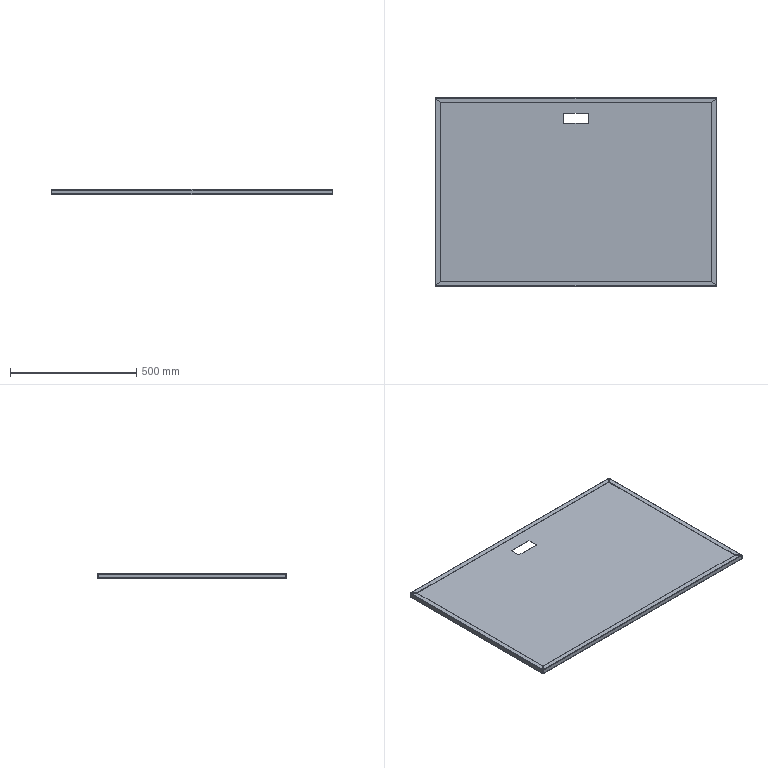Part | SolidWorks | features EdgeFlange 2, FlatPattern 1, ICE 1, SMBaseFlange 1, SheetMetal 1 | 1 solid | 74 faces | box 1116 x 747 x 20 mm | volume 1155364 mm3 | plane 42 | spline 16 | cylinder 16 | commonest cylinder face diameters 2 x8 4.4 x8